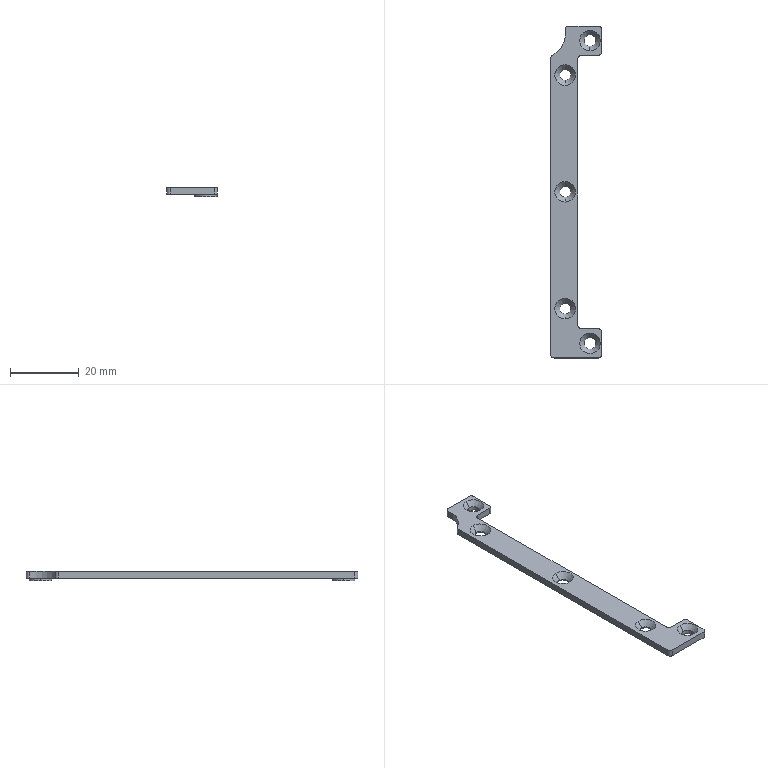NC program | NX | posted with a generic post | part box 14.723 x 96.5 x 2.7 mm
Whole program:
N10 G17 G21 G94 G90
(FLOOR_WALL_COPY , TOOL : D6)
N12 T06 M6
N14 G54
N16 G17 G0 G90 X-59.25 Y7.358 S9500 M3
N18 G43 Z30. H6
N20 Z4.84
N22 G94 G1 Z1.84 F1500.
N24 X-51.25
N26 X51.25
N28 Y4.894
N30 X-51.25
N32 Y2.43
N34 X51.25
N36 Y-0.033
N38 X-51.25
N40 Y-1.167
N42 Y-2.497
N44 X51.25
N46 Y-4.961
N48 X-51.25
N50 X-59.25
N52 Z4.84
N54 G0 Z30.
N56 Y7.358
N58 Z4.38
N60 G1 Z1.38
N62 X-51.25
N64 X51.25
N66 Y4.894
N68 X-51.25
N70 Y2.43
N72 X51.25
N74 Y-0.033
N76 X-51.25
N78 Y-1.167
N80 Y-2.497
N82 X51.25
N84 Y-4.961
N86 X-51.25
N88 X-59.25
N90 Z4.38
N92 G0 Z30.
N94 Y7.358
N96 Z3.92
N98 G1 Z0.92
N100 X-51.25
N102 X51.25
N104 Y4.894
N106 X-51.25
N108 Y2.43
N110 X51.25
N112 Y-0.033
N114 X-51.25
N116 Y-1.167
N118 Y-2.497
N120 X51.25
N122 Y-4.961
N124 X-51.25
N126 X-59.25
N128 Z3.92
N130 G0 Z30.
N132 Y7.358
N134 Z3.46
N136 G1 Z0.46
N138 X-51.25
N140 X51.25
N142 Y4.894
N144 X-51.25
N146 Y2.43
N148 X51.25
N150 Y-0.033
N152 X-51.25
N154 Y-1.167
N156 Y-2.497
N158 X51.25
N160 Y-4.961
N162 X-51.25
N164 X-59.25
N166 Z3.46
N168 G0 Z30.
N170 Y7.358
N172 Z3.
N174 G1 Z0.
N176 X-51.25
N178 X51.25
N180 Y4.894
N182 X-51.25
N184 Y2.43
N186 X51.25
N188 Y-0.033
N190 X-51.25
N192 Y-1.167
N194 Y-2.497
N196 X51.25
N198 Y-4.961
N200 X-51.25
N202 X-59.25
N204 Z3.
N206 G0 Z30.
N208 M5
(FLOOR_WALL_1 , TOOL : D4)
N210 T04 M6
N212 G54
N214 G17 G0 G90 X1.097 Y-10.861 S9500 M3
N216 G43 Z30. H4
N218 Z1.2
N220 G94 G1 Z-0.3 F1000.
N222 X0.346 Y-9.561
N224 G3 X0. Y-9.361 R0.4
N226 G1 X-47.25 F2500.
N228 G2 X-50.25 Y-6.361 R3.
N230 G1 Y6.561
N232 G2 X-47.45 Y9.361 R2.8
N234 G1 X-45.084 Y9.351
N236 G3 X-42.916 Y9.351 R-5.4
N238 G1 X-40.55 Y9.361
N240 G2 X-37.75 Y6.561 R2.8
N242 G1 Y2.561
N244 X37.75
N246 Y6.561
N248 G2 X40.55 Y9.361 R2.8
N250 G1 X42.916 Y9.351
N252 G3 X45.521 Y-1.12 R-5.4
N254 G1 X47.466 Y-2.713
N256 X45.521 Y-1.12
N258 G3 X45.084 Y9.351 R5.4
N260 G1 X47.45 Y9.361
N262 G2 X50.25 Y6.561 R2.8
N264 G1 Y-2.111
N266 G2 X46.857 Y-5.085 R3.
N268 G3 X41.429 Y-7.818 R5.4
N270 G2 X38.806 Y-9.361 R3.
N272 G1 X0.
N274 Y-6.561
N276 X-47.25
N278 G2 X-47.45 Y-6.361 R0.2
N280 G1 Y-3.378
N282 G3 X-37.018 Y-0.239 R8.2
N284 G1 X37.018
N286 G3 X41.438 Y-3.728 R8.2
N288 G1 X43.622 Y-3.404
N290 X41.438 Y-3.728
N292 G3 X38.981 Y-6.458 R8.2
N294 G2 X38.806 Y-6.561 R0.2
N296 G1 X0.
N298 Y-3.761
N300 X-36.266
N302 X-38.28 Y-4.482
N304 X-36.266 Y-3.761
N306 G3 X-35.598 Y-3.039 R11.
N308 G1 X35.598
N310 G3 X36.266 Y-3.761 R11.
N312 G1 X0.
N314 G3 X-0.346 Y-3.961 R0.4
N316 G1 Z1.2
N318 G0 Z30.
N320 X1.097 Y-10.861
N322 Z0.9
N324 G1 Z-0.6 F1000.
N326 X0.346 Y-9.561
N328 G3 X0. Y-9.361 R0.4
N330 G1 X-47.25 F2500.
N332 G2 X-50.25 Y-6.361 R3.
N334 G1 Y6.561
N336 G2 X-47.45 Y9.361 R2.8
N338 G1 X-45.084 Y9.351
N340 G3 X-42.916 Y9.351 R-5.4
N342 G1 X-40.55 Y9.361
N344 G2 X-37.75 Y6.561 R2.8
N346 G1 Y2.561
N348 X37.75
N350 Y6.561
N352 G2 X40.55 Y9.361 R2.8
N354 G1 X42.916 Y9.351
N356 G3 X45.521 Y-1.12 R-5.4
N358 G1 X47.466 Y-2.713
N360 X45.521 Y-1.12
N362 G3 X45.084 Y9.351 R5.4
N364 G1 X47.45 Y9.361
N366 G2 X50.25 Y6.561 R2.8
N368 G1 Y-2.111
N370 G2 X46.857 Y-5.085 R3.
N372 G3 X41.429 Y-7.818 R5.4
N374 G2 X38.806 Y-9.361 R3.
N376 G1 X0.
N378 Y-6.561
N380 X-47.25
N382 G2 X-47.45 Y-6.361 R0.2
N384 G1 Y-3.378
N386 G3 X-37.018 Y-0.239 R8.2
N388 G1 X37.018
N390 G3 X41.438 Y-3.728 R8.2
N392 G1 X43.622 Y-3.404
N394 X41.438 Y-3.728
N396 G3 X38.981 Y-6.458 R8.2
N398 G2 X38.806 Y-6.561 R0.2
N400 G1 X0.
N402 Y-3.761
N404 X-36.266
N406 X-38.28 Y-4.482
N408 X-36.266 Y-3.761
N410 G3 X-35.598 Y-3.039 R11.
N412 G1 X35.598
N414 G3 X36.266 Y-3.761 R11.
N416 G1 X0.
N418 G3 X-0.346 Y-3.961 R0.4
N420 G1 Z0.9
N422 G0 Z30.
(FLOOR_WALL_1_COPY , TOOL : D4)
N424 X-51.75 Y2.913
N426 Z0.8
N428 G1 Z-0.7 F1000.
N430 X-50.599 Y0.971
N432 G3 X-50.25 Y0.775 R0.4
N434 G1 X-48.426 Y0.796 F1200.
N436 G3 X-45.986 Y-1.068 R5.5
N438 G1 X-50.25 Y-1.117
N440 G2 X-50.599 Y-0.921 R0.4
N442 G1 X-51.75 Y1.021
N444 Z0.8
N446 G0 Z30.
N448 X-36.25 Y4.061
N450 Z0.8
N452 G1 Z-0.7 F1000.
N454 X-39.137 Y1.068
N456 G3 X-39.5 Y0.899 R0.4
N458 G1 X38.983 Y1.808 F1200.
N460 G3 X40.366 Y-0.068 R5.5
N462 G1 X-41.895 Y-1.02
N464 Z0.8
N466 G0 Z30.
N468 X51.75 Y2.463
N470 Z0.8
N472 G1 Z-0.7 F1000.
N474 X49.387 Y2.166
N476 G3 X49.068 Y1.925 R0.4
N478 G1 X50.25 Y1.939 F1200.
N480 Y0.047
N482 X47.728 Y0.018
N484 Z0.8
N486 G0 Z30.
N488 X-51.75 Y-0.871
N490 Z0.8
N492 G1 Z-0.7 F1000.
N494 X-50.599 Y-2.813
N496 G3 X-50.25 Y-3.009 R0.4
N498 G1 X50.25 Y-1.845 F1200.
N500 Y-2.111
N502 G2 X49.768 Y-3.742 R3.
N504 G1 X-50.25 Y-4.901
N506 Y-6.361
N508 G3 X-50.219 Y-6.792 R3.
N510 G1 X43.549 Y-5.706
N512 G3 X43.893 Y-5.502 R0.4
N514 G1 X44.529 Y-6.892
N516 Z0.8
N518 G0 Z30.
N520 X43.35 Y10.861
N522 Z0.8
N524 G1 Z-0.7 F1000.
N526 X43.992 Y9.572
N528 G3 X44.325 Y9.351 R0.4
N530 G2 X43.675 Y9.351 R-5.3 F1200.
N532 G3 X44.008 Y9.572 R0.4
N534 G1 X44.65 Y10.861
N536 Z0.8
N538 G0 Z30.
N540 X-44.65
N542 Z0.8
N544 G1 Z-0.7 F1000.
N546 X-44.008 Y9.572
N548 G3 X-43.675 Y9.351 R0.4
N550 G2 X-44.325 Y9.351 R-5.3 F1200.
N552 G3 X-43.992 Y9.572 R0.4
N554 G1 X-43.35 Y10.861
N556 Z0.8
N558 G0 Z30.
N560 M5
(PLANAR_MILL_COPY , TOOL : D6A45)
N562 T07 M6
N564 G54
N566 G17 G0 G90 X-43.134 Y4.861 S9500 M3
N568 G43 Z30. H7
N570 Z1.
N572 G94 G1 Z-0.5 F1250.
N574 G3 X-44. Y5.361 R1.
N576 X-45.3 Y4.061 R1.3
N578 X-44. Y5.361 R-1.3
N580 X-44.866 Y4.861 R1.
N582 G1 Z1.
N584 G0 Z30.
N586 Y8.261
N588 Z1.
N590 G1 Z-0.5
N592 G3 X-44. Y7.761 R1.
N594 G2 X-40.3 Y4.061 R3.7
N596 X-44. Y7.761 R-3.7
N598 G3 X-43.134 Y8.261 R1.
N600 G1 Z1.
N602 G0 Z30.
N604 X44.866 Y4.861
N606 Z1.
N608 G1 Z-0.5
N610 G3 X44. Y5.361 R1.
N612 X42.7 Y4.061 R1.3
N614 X44. Y5.361 R-1.3
N616 X43.134 Y4.861 R1.
N618 G1 Z1.
N620 G0 Z30.
N622 Y8.261
N624 Z1.
N626 G1 Z-0.5
N628 G3 X44. Y7.761 R1.
N630 G2 X47.7 Y4.061 R3.7
N632 X44. Y7.761 R-3.7
N634 G3 X44.866 Y8.261 R1.
N636 G1 Z1.
N638 G0 Z30.
(PLANAR_MILL_COPY_COPY , TOOL : D6A45)
N640 X33.3 Y-3.092
N642 Z-0.2
N644 G1 Y-3.269 Z-0.247
N646 X33.406 Y-3.539 Z-0.325
N648 X33.611 Y-3.744 Z-0.403
N650 X33.881 Y-3.85 Z-0.481
N652 X34.119 Z-0.544
N654 X34.389 Y-3.744 Z-0.622
N656 X34.594 Y-3.539 Z-0.7
N658 X34.7 Y-3.269 Z-0.778
N660 Y-3.031 Z-0.841
N662 X34.594 Y-2.761 Z-0.919
N664 X34.389 Y-2.556 Z-0.997
N666 X34.119 Y-2.45 Z-1.074
N668 X33.881 Z-1.138
N670 X33.611 Y-2.556 Z-1.216
N672 X33.406 Y-2.761 Z-1.294
N674 X33.3 Y-3.031 Z-1.371
N676 Y-3.269 Z-1.435
N678 X33.406 Y-3.539 Z-1.513
N680 X33.611 Y-3.744 Z-1.59
N682 X33.881 Y-3.85 Z-1.668
N684 X34. Z-1.7
N686 G3 X34.7 Y-3.15 R0.7
N688 X34. Y-3.85 R-0.7
N690 X34.433 Y-3.6 R0.5
N692 G1 Z-0.2
N694 G0 Z30.
N696 X37.405 Y5.245
N698 Z-0.2
N700 G1 Z-1.7
N702 X38.078 Y5.357
N704 G3 X38.85 Y5.992 R1.
N706 G1 Y6.561
N708 G2 X40.445 Y8.258 R1.7
N710 G3 X40.783 Y9.199 R1.
N712 G1 X40.661 Y9.87
N714 Z-0.2
N716 G0 Z30.
N718 X47.339
N720 Z-0.2
N722 G1 Z-1.7
N724 X47.217 Y9.199
N726 G3 X47.555 Y8.258 R1.
N728 G2 X49.15 Y6.561 R1.7
N730 G1 Y5.992
N732 G3 X49.922 Y5.357 R1.
N734 G1 Y2.766
N736 G3 X49.15 Y2.131 R1.
N738 G1 Y-2.111
N740 G2 X47.001 Y-3.995 R1.9
N742 G3 X40.467 Y-7.284 R6.5
N744 G2 X38.806 Y-8.261 R1.9
N746 G1 X-47.25
N748 G2 X-49.15 Y-6.361 R1.9
N750 G1 Y2.131
N752 G3 X-49.922 Y2.766 R1.
N754 G1 Y5.357
N756 G3 X-49.15 Y5.992 R1.
N758 G1 Y6.561
N760 G2 X-47.555 Y8.258 R1.7
N762 G3 X-47.217 Y9.199 R1.
N764 G1 X-47.339 Y9.87
N766 Z-0.2
N768 G0 Z30.
N770 X-40.661
N772 Z-0.2
N774 G1 Z-1.7
N776 X-40.783 Y9.199
N778 G3 X-40.445 Y8.258 R1.
N780 G2 X-38.85 Y6.561 R1.7
N782 G1 Y5.992
N784 G3 X-38.078 Y5.357 R1.
N786 G1 Y2.766
N788 G3 X-38.85 Y2.131 R1.
N790 G1 Y1.561
N792 X-38.845 Y1.506
N794 X-38.805 Y1.466
N796 X-38.75 Y1.461
N798 X38.75
N800 X38.805 Y1.466
N802 X38.845 Y1.506
N804 X38.85 Y1.561
N806 Y2.131
N808 G3 X38.078 Y2.766 R1.
N810 G1 X37.405 Y2.878
N812 Z-0.2
N814 G0 Z30.
N816 X0.75 Y-3.208
N818 Z-0.2
N820 G1 Y-3.031 Z-0.247
N822 X0.644 Y-2.761 Z-0.325
N824 X0.439 Y-2.556 Z-0.403
N826 X0.169 Y-2.45 Z-0.481
N828 X-0.069 Z-0.544
N830 X-0.339 Y-2.556 Z-0.622
N832 X-0.544 Y-2.761 Z-0.7
N834 X-0.65 Y-3.031 Z-0.778
N836 Y-3.269 Z-0.841
N838 X-0.544 Y-3.539 Z-0.919
N840 X-0.339 Y-3.744 Z-0.997
N842 X-0.069 Y-3.85 Z-1.074
N844 X0.169 Z-1.138
N846 X0.439 Y-3.744 Z-1.216
N848 X0.644 Y-3.539 Z-1.294
N850 X0.75 Y-3.269 Z-1.371
N852 Y-3.031 Z-1.435
N854 X0.644 Y-2.761 Z-1.513
N856 X0.439 Y-2.556 Z-1.59
N858 X0.169 Y-2.45 Z-1.668
N860 X0.05 Z-1.7
N862 G3 X-0.65 Y-3.15 R0.7
N864 X0.05 Y-2.45 R-0.7
N866 X-0.383 Y-2.7 R0.5
N868 G1 Z-0.2
N870 G0 Z30.
N872 X-34.6 Y-3.092
N874 Z-0.2
N876 G1 Y-3.269 Z-0.247
N878 X-34.494 Y-3.539 Z-0.325
N880 X-34.289 Y-3.744 Z-0.403
N882 X-34.019 Y-3.85 Z-0.481
N884 X-33.781 Z-0.544
N886 X-33.511 Y-3.744 Z-0.622
N888 X-33.306 Y-3.539 Z-0.7
N890 X-33.2 Y-3.269 Z-0.778
N892 Y-3.031 Z-0.841
N894 X-33.306 Y-2.761 Z-0.919
N896 X-33.511 Y-2.556 Z-0.997
N898 X-33.781 Y-2.45 Z-1.074
N900 X-34.019 Z-1.138
N902 X-34.289 Y-2.556 Z-1.216
N904 X-34.494 Y-2.761 Z-1.294
N906 X-34.6 Y-3.031 Z-1.371
N908 Y-3.269 Z-1.435
N910 X-34.494 Y-3.539 Z-1.513
N912 X-34.289 Y-3.744 Z-1.59
N914 X-34.019 Y-3.85 Z-1.668
N916 X-33.9 Z-1.7
N918 G3 X-33.2 Y-3.15 R0.7
N920 X-33.9 Y-3.85 R-0.7
N922 X-33.467 Y-3.6 R0.5
N924 G1 Z-0.2
N926 G0 Z30.
N928 M5
N930 M2